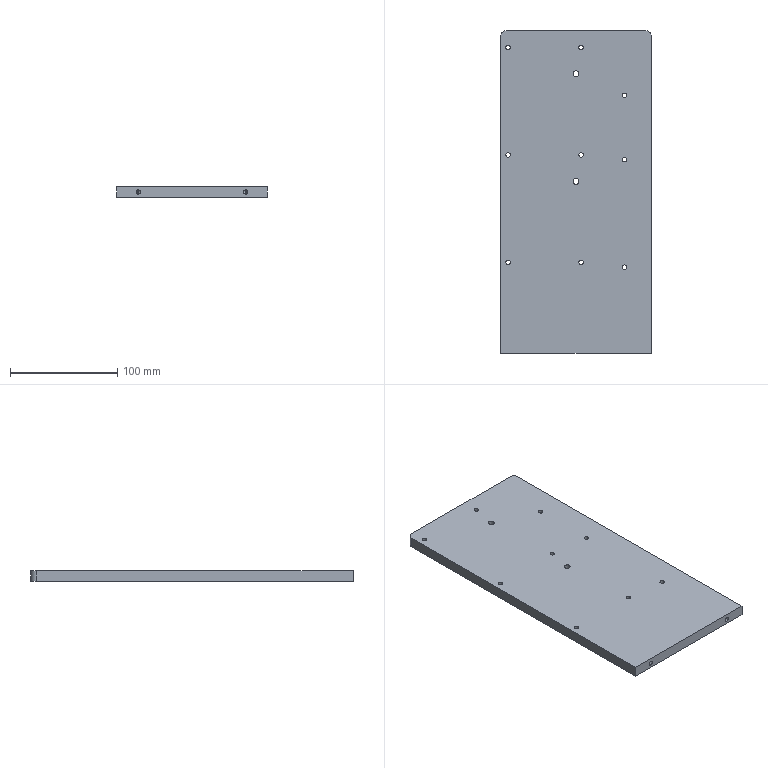Part | SolidWorks | features HoleWzd 4, Extrusion 1, Fillet 1 | 1 solid | 44 faces | box 140 x 300 x 10 mm | volume 417191 mm3 | cylinder 32 | plane 8 | cone 4 | commonest cylinder face diameters 4.2 x22 10 x6 5.5 x4
STEP:
#1=CARTESIAN_POINT('',(42.9,90.,0.));
#2=VERTEX_POINT('',#1);
#3=CARTESIAN_POINT('',(47.1,90.,0.));
#4=VERTEX_POINT('',#3);
#5=CARTESIAN_POINT('',(45.,90.,0.));
#6=DIRECTION('',(0.,0.,1.));
#7=DIRECTION('',(1.,0.,0.));
#8=AXIS2_PLACEMENT_3D('',#5,#6,#7);
#9=CIRCLE('',#8,2.1);
#10=EDGE_CURVE('',#2,#4,#9,.T.);
#11=ORIENTED_EDGE('',*,*,#10,.F.);
#12=CARTESIAN_POINT('',(42.9,90.,10.));
#13=VERTEX_POINT('',#12);
#14=CARTESIAN_POINT('',(42.9,90.,10.));
#15=DIRECTION('',(0.,0.,1.));
#16=VECTOR('',#15,1000.);
#17=LINE('',#14,#16);
#18=EDGE_CURVE('',#2,#13,#17,.T.);
#19=ORIENTED_EDGE('',*,*,#18,.T.);
#20=CARTESIAN_POINT('',(47.1,90.,10.));
#21=VERTEX_POINT('',#20);
#22=CARTESIAN_POINT('',(45.,90.,10.));
#23=DIRECTION('',(0.,0.,1.));
#24=DIRECTION('',(1.,0.,0.));
#25=AXIS2_PLACEMENT_3D('',#22,#23,#24);
#26=CIRCLE('',#25,2.1);
#27=EDGE_CURVE('',#13,#21,#26,.T.);
#28=ORIENTED_EDGE('',*,*,#27,.T.);
#29=CARTESIAN_POINT('',(47.1,90.,10.));
#30=DIRECTION('',(0.,0.,1.));
#31=VECTOR('',#30,1000.);
#32=LINE('',#29,#31);
#33=EDGE_CURVE('',#4,#21,#32,.T.);
#34=ORIENTED_EDGE('',*,*,#33,.F.);
#35=EDGE_LOOP('',(#11,#19,#28,#34));
#36=FACE_OUTER_BOUND('',#35,.T.);
#37=CARTESIAN_POINT('',(45.,90.,10.));
#38=DIRECTION('',(0.,0.,1.));
#39=DIRECTION('',(1.,0.,0.));
#40=AXIS2_PLACEMENT_3D('',#37,#38,#39);
#41=CYLINDRICAL_SURFACE('',#40,2.1);
#42=ADVANCED_FACE('',(#36),#41,.F.);
#43=CARTESIAN_POINT('',(42.9,30.,0.));
#44=VERTEX_POINT('',#43);
#45=CARTESIAN_POINT('',(47.1,30.,0.));
#46=VERTEX_POINT('',#45);
#47=CARTESIAN_POINT('',(45.,30.,0.));
#48=DIRECTION('',(0.,0.,1.));
#49=DIRECTION('',(1.,0.,0.));
#50=AXIS2_PLACEMENT_3D('',#47,#48,#49);
#51=CIRCLE('',#50,2.1);
#52=EDGE_CURVE('',#44,#46,#51,.T.);
#53=ORIENTED_EDGE('',*,*,#52,.F.);
#54=CARTESIAN_POINT('',(42.9,30.,10.));
#55=VERTEX_POINT('',#54);
#56=CARTESIAN_POINT('',(42.9,30.,10.));
#57=DIRECTION('',(0.,0.,1.));
#58=VECTOR('',#57,1000.);
#59=LINE('',#56,#58);
#60=EDGE_CURVE('',#44,#55,#59,.T.);
#61=ORIENTED_EDGE('',*,*,#60,.T.);
#62=CARTESIAN_POINT('',(47.1,30.,10.));
#63=VERTEX_POINT('',#62);
#64=CARTESIAN_POINT('',(45.,30.,10.));
#65=DIRECTION('',(0.,0.,1.));
#66=DIRECTION('',(1.,0.,0.));
#67=AXIS2_PLACEMENT_3D('',#64,#65,#66);
#68=CIRCLE('',#67,2.1);
#69=EDGE_CURVE('',#55,#63,#68,.T.);
#70=ORIENTED_EDGE('',*,*,#69,.T.);
#71=CARTESIAN_POINT('',(47.1,30.,10.));
#72=DIRECTION('',(0.,0.,1.));
#73=VECTOR('',#72,1000.);
#74=LINE('',#71,#73);
#75=EDGE_CURVE('',#46,#63,#74,.T.);
#76=ORIENTED_EDGE('',*,*,#75,.F.);
#77=EDGE_LOOP('',(#53,#61,#70,#76));
#78=FACE_OUTER_BOUND('',#77,.T.);
#79=CARTESIAN_POINT('',(45.,30.,10.));
#80=DIRECTION('',(0.,0.,1.));
#81=DIRECTION('',(1.,0.,0.));
#82=AXIS2_PLACEMENT_3D('',#79,#80,#81);
#83=CYLINDRICAL_SURFACE('',#82,2.1);
#84=ADVANCED_FACE('',(#78),#83,.F.);
#85=CARTESIAN_POINT('',(42.9,-70.,0.));
#86=VERTEX_POINT('',#85);
#87=CARTESIAN_POINT('',(47.1,-70.,0.));
#88=VERTEX_POINT('',#87);
#89=CARTESIAN_POINT('',(45.,-70.,0.));
#90=DIRECTION('',(0.,0.,1.));
#91=DIRECTION('',(1.,0.,0.));
#92=AXIS2_PLACEMENT_3D('',#89,#90,#91);
#93=CIRCLE('',#92,2.1);
#94=EDGE_CURVE('',#86,#88,#93,.T.);
#95=ORIENTED_EDGE('',*,*,#94,.F.);
#96=CARTESIAN_POINT('',(42.9,-70.,10.));
#97=VERTEX_POINT('',#96);
#98=CARTESIAN_POINT('',(42.9,-70.,10.));
#99=DIRECTION('',(0.,0.,1.));
#100=VECTOR('',#99,1000.);
#101=LINE('',#98,#100);
#102=EDGE_CURVE('',#86,#97,#101,.T.);
#103=ORIENTED_EDGE('',*,*,#102,.T.);
#104=CARTESIAN_POINT('',(47.1,-70.,10.));
#105=VERTEX_POINT('',#104);
#106=CARTESIAN_POINT('',(45.,-70.,10.));
#107=DIRECTION('',(0.,0.,1.));
#108=DIRECTION('',(1.,0.,0.));
#109=AXIS2_PLACEMENT_3D('',#106,#107,#108);
#110=CIRCLE('',#109,2.1);
#111=EDGE_CURVE('',#97,#105,#110,.T.);
#112=ORIENTED_EDGE('',*,*,#111,.T.);
#113=CARTESIAN_POINT('',(47.1,-70.,10.));
#114=DIRECTION('',(0.,0.,1.));
#115=VECTOR('',#114,1000.);
#116=LINE('',#113,#115);
#117=EDGE_CURVE('',#88,#105,#116,.T.);
#118=ORIENTED_EDGE('',*,*,#117,.F.);
#119=EDGE_LOOP('',(#95,#103,#112,#118));
#120=FACE_OUTER_BOUND('',#119,.T.);
#121=CARTESIAN_POINT('',(45.,-70.,10.));
#122=DIRECTION('',(0.,0.,1.));
#123=DIRECTION('',(1.,0.,0.));
#124=AXIS2_PLACEMENT_3D('',#121,#122,#123);
#125=CYLINDRICAL_SURFACE('',#124,2.1);
#126=ADVANCED_FACE('',(#120),#125,.F.);
#127=CARTESIAN_POINT('',(50.,-137.6,7.1));
#128=VERTEX_POINT('',#127);
#129=CARTESIAN_POINT('',(50.,-137.6,2.9));
#130=VERTEX_POINT('',#129);
#131=CARTESIAN_POINT('',(50.,-137.6,5.));
#132=DIRECTION('',(0.,-1.,0.));
#133=DIRECTION('',(0.,0.,-1.));
#134=AXIS2_PLACEMENT_3D('',#131,#132,#133);
#135=CIRCLE('',#134,2.1);
#136=EDGE_CURVE('',#128,#130,#135,.T.);
#137=ORIENTED_EDGE('',*,*,#136,.F.);
#138=CARTESIAN_POINT('',(50.,-150.,7.1));
#139=VERTEX_POINT('',#138);
#140=CARTESIAN_POINT('',(50.,-150.,7.1));
#141=DIRECTION('',(0.,-1.,0.));
#142=VECTOR('',#141,1000.);
#143=LINE('',#140,#142);
#144=EDGE_CURVE('',#128,#139,#143,.T.);
#145=ORIENTED_EDGE('',*,*,#144,.T.);
#146=CARTESIAN_POINT('',(50.,-150.,2.9));
#147=VERTEX_POINT('',#146);
#148=CARTESIAN_POINT('',(50.,-150.,5.));
#149=DIRECTION('',(0.,-1.,0.));
#150=DIRECTION('',(0.,0.,-1.));
#151=AXIS2_PLACEMENT_3D('',#148,#149,#150);
#152=CIRCLE('',#151,2.1);
#153=EDGE_CURVE('',#139,#147,#152,.T.);
#154=ORIENTED_EDGE('',*,*,#153,.T.);
#155=CARTESIAN_POINT('',(50.,-150.,2.9));
#156=DIRECTION('',(0.,-1.,0.));
#157=VECTOR('',#156,1000.);
#158=LINE('',#155,#157);
#159=EDGE_CURVE('',#130,#147,#158,.T.);
#160=ORIENTED_EDGE('',*,*,#159,.F.);
#161=EDGE_LOOP('',(#137,#145,#154,#160));
#162=FACE_OUTER_BOUND('',#161,.T.);
#163=CARTESIAN_POINT('',(50.,-150.,5.));
#164=DIRECTION('',(0.,-1.,0.));
#165=DIRECTION('',(0.,0.,-1.));
#166=AXIS2_PLACEMENT_3D('',#163,#164,#165);
#167=CYLINDRICAL_SURFACE('',#166,2.1);
#168=ADVANCED_FACE('',(#162),#167,.F.);
#169=CARTESIAN_POINT('',(50.,-136.338,5.));
#170=VERTEX_POINT('',#169);
#171=CARTESIAN_POINT('',(50.,-137.6,2.9));
#172=DIRECTION('',(0.,-0.515,-0.8572));
#173=VECTOR('',#172,1000.);
#174=LINE('',#171,#173);
#175=EDGE_CURVE('',#170,#130,#174,.T.);
#176=ORIENTED_EDGE('',*,*,#175,.F.);
#177=CARTESIAN_POINT('',(50.,-137.6,7.1));
#178=DIRECTION('',(0.,-0.515,0.8572));
#179=VECTOR('',#178,1000.);
#180=LINE('',#177,#179);
#181=EDGE_CURVE('',#170,#128,#180,.T.);
#182=ORIENTED_EDGE('',*,*,#181,.T.);
#183=ORIENTED_EDGE('',*,*,#136,.T.);
#184=EDGE_LOOP('',(#176,#182,#183));
#185=FACE_OUTER_BOUND('',#184,.T.);
#186=CARTESIAN_POINT('',(50.,-137.6,5.));
#187=DIRECTION('',(0.,-1.,0.));
#188=DIRECTION('',(0.,0.,-1.));
#189=AXIS2_PLACEMENT_3D('',#186,#187,#188);
#190=CONICAL_SURFACE('',#189,2.1,1.03);
#191=ADVANCED_FACE('',(#185),#190,.F.);
#192=CARTESIAN_POINT('',(-50.,-137.6,7.1));
#193=VERTEX_POINT('',#192);
#194=CARTESIAN_POINT('',(-50.,-137.6,2.9));
#195=VERTEX_POINT('',#194);
#196=CARTESIAN_POINT('',(-50.,-137.6,5.));
#197=DIRECTION('',(0.,-1.,0.));
#198=DIRECTION('',(0.,0.,-1.));
#199=AXIS2_PLACEMENT_3D('',#196,#197,#198);
#200=CIRCLE('',#199,2.1);
#201=EDGE_CURVE('',#193,#195,#200,.T.);
#202=ORIENTED_EDGE('',*,*,#201,.F.);
#203=CARTESIAN_POINT('',(-50.,-150.,7.1));
#204=VERTEX_POINT('',#203);
#205=CARTESIAN_POINT('',(-50.,-150.,7.1));
#206=DIRECTION('',(0.,-1.,0.));
#207=VECTOR('',#206,1000.);
#208=LINE('',#205,#207);
#209=EDGE_CURVE('',#193,#204,#208,.T.);
#210=ORIENTED_EDGE('',*,*,#209,.T.);
#211=CARTESIAN_POINT('',(-50.,-150.,2.9));
#212=VERTEX_POINT('',#211);
#213=CARTESIAN_POINT('',(-50.,-150.,5.));
#214=DIRECTION('',(0.,-1.,0.));
#215=DIRECTION('',(0.,0.,-1.));
#216=AXIS2_PLACEMENT_3D('',#213,#214,#215);
#217=CIRCLE('',#216,2.1);
#218=EDGE_CURVE('',#204,#212,#217,.T.);
#219=ORIENTED_EDGE('',*,*,#218,.T.);
#220=CARTESIAN_POINT('',(-50.,-150.,2.9));
#221=DIRECTION('',(0.,-1.,0.));
#222=VECTOR('',#221,1000.);
#223=LINE('',#220,#222);
#224=EDGE_CURVE('',#195,#212,#223,.T.);
#225=ORIENTED_EDGE('',*,*,#224,.F.);
#226=EDGE_LOOP('',(#202,#210,#219,#225));
#227=FACE_OUTER_BOUND('',#226,.T.);
#228=CARTESIAN_POINT('',(-50.,-150.,5.));
#229=DIRECTION('',(0.,-1.,0.));
#230=DIRECTION('',(0.,0.,-1.));
#231=AXIS2_PLACEMENT_3D('',#228,#229,#230);
#232=CYLINDRICAL_SURFACE('',#231,2.1);
#233=ADVANCED_FACE('',(#227),#232,.F.);
#234=CARTESIAN_POINT('',(-50.,-136.338,5.));
#235=VERTEX_POINT('',#234);
#236=CARTESIAN_POINT('',(-50.,-137.6,2.9));
#237=DIRECTION('',(0.,-0.515,-0.8572));
#238=VECTOR('',#237,1000.);
#239=LINE('',#236,#238);
#240=EDGE_CURVE('',#235,#195,#239,.T.);
#241=ORIENTED_EDGE('',*,*,#240,.F.);
#242=CARTESIAN_POINT('',(-50.,-137.6,7.1));
#243=DIRECTION('',(0.,-0.515,0.8572));
#244=VECTOR('',#243,1000.);
#245=LINE('',#242,#244);
#246=EDGE_CURVE('',#235,#193,#245,.T.);
#247=ORIENTED_EDGE('',*,*,#246,.T.);
#248=ORIENTED_EDGE('',*,*,#201,.T.);
#249=EDGE_LOOP('',(#241,#247,#248));
#250=FACE_OUTER_BOUND('',#249,.T.);
#251=CARTESIAN_POINT('',(-50.,-137.6,5.));
#252=DIRECTION('',(0.,-1.,0.));
#253=DIRECTION('',(0.,0.,-1.));
#254=AXIS2_PLACEMENT_3D('',#251,#252,#253);
#255=CONICAL_SURFACE('',#254,2.1,1.03);
#256=ADVANCED_FACE('',(#250),#255,.F.);
#257=CARTESIAN_POINT('',(2.7,-65.5,10.));
#258=VERTEX_POINT('',#257);
#259=CARTESIAN_POINT('',(6.9,-65.5,10.));
#260=VERTEX_POINT('',#259);
#261=CARTESIAN_POINT('',(4.8,-65.5,10.));
#262=DIRECTION('',(0.,0.,1.));
#263=DIRECTION('',(1.,0.,0.));
#264=AXIS2_PLACEMENT_3D('',#261,#262,#263);
#265=CIRCLE('',#264,2.1);
#266=EDGE_CURVE('',#258,#260,#265,.T.);
#267=ORIENTED_EDGE('',*,*,#266,.T.);
#268=CARTESIAN_POINT('',(6.9,-65.5,0.));
#269=VERTEX_POINT('',#268);
#270=CARTESIAN_POINT('',(6.9,-65.5,0.));
#271=DIRECTION('',(0.,0.,-1.));
#272=VECTOR('',#271,1000.);
#273=LINE('',#270,#272);
#274=EDGE_CURVE('',#260,#269,#273,.T.);
#275=ORIENTED_EDGE('',*,*,#274,.T.);
#276=CARTESIAN_POINT('',(2.7,-65.5,0.));
#277=VERTEX_POINT('',#276);
#278=CARTESIAN_POINT('',(4.8,-65.5,0.));
#279=DIRECTION('',(0.,0.,-1.));
#280=DIRECTION('',(-1.,0.,0.));
#281=AXIS2_PLACEMENT_3D('',#278,#279,#280);
#282=CIRCLE('',#281,2.1);
#283=EDGE_CURVE('',#269,#277,#282,.T.);
#284=ORIENTED_EDGE('',*,*,#283,.T.);
#285=CARTESIAN_POINT('',(2.7,-65.5,0.));
#286=DIRECTION('',(0.,0.,-1.));
#287=VECTOR('',#286,1000.);
#288=LINE('',#285,#287);
#289=EDGE_CURVE('',#258,#277,#288,.T.);
#290=ORIENTED_EDGE('',*,*,#289,.F.);
#291=EDGE_LOOP('',(#267,#275,#284,#290));
#292=FACE_OUTER_BOUND('',#291,.T.);
#293=CARTESIAN_POINT('',(4.8,-65.5,0.));
#294=DIRECTION('',(0.,0.,-1.));
#295=DIRECTION('',(-1.,0.,0.));
#296=AXIS2_PLACEMENT_3D('',#293,#294,#295);
#297=CYLINDRICAL_SURFACE('',#296,2.1);
#298=ADVANCED_FACE('',(#292),#297,.F.);
#299=CARTESIAN_POINT('',(-65.3,-65.5,10.));
#300=VERTEX_POINT('',#299);
#301=CARTESIAN_POINT('',(-61.1,-65.5,10.));
#302=VERTEX_POINT('',#301);
#303=CARTESIAN_POINT('',(-63.2,-65.5,10.));
#304=DIRECTION('',(0.,0.,1.));
#305=DIRECTION('',(1.,0.,0.));
#306=AXIS2_PLACEMENT_3D('',#303,#304,#305);
#307=CIRCLE('',#306,2.1);
#308=EDGE_CURVE('',#300,#302,#307,.T.);
#309=ORIENTED_EDGE('',*,*,#308,.T.);
#310=CARTESIAN_POINT('',(-61.1,-65.5,0.));
#311=VERTEX_POINT('',#310);
#312=CARTESIAN_POINT('',(-61.1,-65.5,0.));
#313=DIRECTION('',(0.,0.,-1.));
#314=VECTOR('',#313,1000.);
#315=LINE('',#312,#314);
#316=EDGE_CURVE('',#302,#311,#315,.T.);
#317=ORIENTED_EDGE('',*,*,#316,.T.);
#318=CARTESIAN_POINT('',(-65.3,-65.5,0.));
#319=VERTEX_POINT('',#318);
#320=CARTESIAN_POINT('',(-63.2,-65.5,0.));
#321=DIRECTION('',(0.,0.,-1.));
#322=DIRECTION('',(-1.,0.,0.));
#323=AXIS2_PLACEMENT_3D('',#320,#321,#322);
#324=CIRCLE('',#323,2.1);
#325=EDGE_CURVE('',#311,#319,#324,.T.);
#326=ORIENTED_EDGE('',*,*,#325,.T.);
#327=CARTESIAN_POINT('',(-65.3,-65.5,0.));
#328=DIRECTION('',(0.,0.,-1.));
#329=VECTOR('',#328,1000.);
#330=LINE('',#327,#329);
#331=EDGE_CURVE('',#300,#319,#330,.T.);
#332=ORIENTED_EDGE('',*,*,#331,.F.);
#333=EDGE_LOOP('',(#309,#317,#326,#332));
#334=FACE_OUTER_BOUND('',#333,.T.);
#335=CARTESIAN_POINT('',(-63.2,-65.5,0.));
#336=DIRECTION('',(0.,0.,-1.));
#337=DIRECTION('',(-1.,0.,0.));
#338=AXIS2_PLACEMENT_3D('',#335,#336,#337);
#339=CYLINDRICAL_SURFACE('',#338,2.1);
#340=ADVANCED_FACE('',(#334),#339,.F.);
#341=CARTESIAN_POINT('',(2.7,34.5,10.));
#342=VERTEX_POINT('',#341);
#343=CARTESIAN_POINT('',(6.9,34.5,10.));
#344=VERTEX_POINT('',#343);
#345=CARTESIAN_POINT('',(4.8,34.5,10.));
#346=DIRECTION('',(0.,0.,1.));
#347=DIRECTION('',(1.,0.,0.));
#348=AXIS2_PLACEMENT_3D('',#345,#346,#347);
#349=CIRCLE('',#348,2.1);
#350=EDGE_CURVE('',#342,#344,#349,.T.);
#351=ORIENTED_EDGE('',*,*,#350,.T.);
#352=CARTESIAN_POINT('',(6.9,34.5,0.));
#353=VERTEX_POINT('',#352);
#354=CARTESIAN_POINT('',(6.9,34.5,0.));
#355=DIRECTION('',(0.,0.,-1.));
#356=VECTOR('',#355,1000.);
#357=LINE('',#354,#356);
#358=EDGE_CURVE('',#344,#353,#357,.T.);
#359=ORIENTED_EDGE('',*,*,#358,.T.);
#360=CARTESIAN_POINT('',(2.7,34.5,0.));
#361=VERTEX_POINT('',#360);
#362=CARTESIAN_POINT('',(4.8,34.5,0.));
#363=DIRECTION('',(0.,0.,-1.));
#364=DIRECTION('',(-1.,0.,0.));
#365=AXIS2_PLACEMENT_3D('',#362,#363,#364);
#366=CIRCLE('',#365,2.1);
#367=EDGE_CURVE('',#353,#361,#366,.T.);
#368=ORIENTED_EDGE('',*,*,#367,.T.);
#369=CARTESIAN_POINT('',(2.7,34.5,0.));
#370=DIRECTION('',(0.,0.,-1.));
#371=VECTOR('',#370,1000.);
#372=LINE('',#369,#371);
#373=EDGE_CURVE('',#342,#361,#372,.T.);
#374=ORIENTED_EDGE('',*,*,#373,.F.);
#375=EDGE_LOOP('',(#351,#359,#368,#374));
#376=FACE_OUTER_BOUND('',#375,.T.);
#377=CARTESIAN_POINT('',(4.8,34.5,0.));
#378=DIRECTION('',(0.,0.,-1.));
#379=DIRECTION('',(-1.,0.,0.));
#380=AXIS2_PLACEMENT_3D('',#377,#378,#379);
#381=CYLINDRICAL_SURFACE('',#380,2.1);
#382=ADVANCED_FACE('',(#376),#381,.F.);
#383=CARTESIAN_POINT('',(-65.3,34.5,10.));
#384=VERTEX_POINT('',#383);
#385=CARTESIAN_POINT('',(-61.1,34.5,10.));
#386=VERTEX_POINT('',#385);
#387=CARTESIAN_POINT('',(-63.2,34.5,10.));
#388=DIRECTION('',(0.,0.,1.));
#389=DIRECTION('',(1.,0.,0.));
#390=AXIS2_PLACEMENT_3D('',#387,#388,#389);
#391=CIRCLE('',#390,2.1);
#392=EDGE_CURVE('',#384,#386,#391,.T.);
#393=ORIENTED_EDGE('',*,*,#392,.T.);
#394=CARTESIAN_POINT('',(-61.1,34.5,0.));
#395=VERTEX_POINT('',#394);
#396=CARTESIAN_POINT('',(-61.1,34.5,0.));
#397=DIRECTION('',(0.,0.,-1.));
#398=VECTOR('',#397,1000.);
#399=LINE('',#396,#398);
#400=EDGE_CURVE('',#386,#395,#399,.T.);
#401=ORIENTED_EDGE('',*,*,#400,.T.);
#402=CARTESIAN_POINT('',(-65.3,34.5,0.));
#403=VERTEX_POINT('',#402);
#404=CARTESIAN_POINT('',(-63.2,34.5,0.));
#405=DIRECTION('',(0.,0.,-1.));
#406=DIRECTION('',(-1.,0.,0.));
#407=AXIS2_PLACEMENT_3D('',#404,#405,#406);
#408=CIRCLE('',#407,2.1);
#409=EDGE_CURVE('',#395,#403,#408,.T.);
#410=ORIENTED_EDGE('',*,*,#409,.T.);
#411=CARTESIAN_POINT('',(-65.3,34.5,0.));
#412=DIRECTION('',(0.,0.,-1.));
#413=VECTOR('',#412,1000.);
#414=LINE('',#411,#413);
#415=EDGE_CURVE('',#384,#403,#414,.T.);
#416=ORIENTED_EDGE('',*,*,#415,.F.);
#417=EDGE_LOOP('',(#393,#401,#410,#416));
#418=FACE_OUTER_BOUND('',#417,.T.);
#419=CARTESIAN_POINT('',(-63.2,34.5,0.));
#420=DIRECTION('',(0.,0.,-1.));
#421=DIRECTION('',(-1.,0.,0.));
#422=AXIS2_PLACEMENT_3D('',#419,#420,#421);
#423=CYLINDRICAL_SURFACE('',#422,2.1);
#424=ADVANCED_FACE('',(#418),#423,.F.);
#425=CARTESIAN_POINT('',(2.7,134.5,10.));
#426=VERTEX_POINT('',#425);
#427=CARTESIAN_POINT('',(6.9,134.5,10.));
#428=VERTEX_POINT('',#427);
#429=CARTESIAN_POINT('',(4.8,134.5,10.));
#430=DIRECTION('',(0.,0.,1.));
#431=DIRECTION('',(1.,0.,0.));
#432=AXIS2_PLACEMENT_3D('',#429,#430,#431);
#433=CIRCLE('',#432,2.1);
#434=EDGE_CURVE('',#426,#428,#433,.T.);
#435=ORIENTED_EDGE('',*,*,#434,.T.);
#436=CARTESIAN_POINT('',(6.9,134.5,0.));
#437=VERTEX_POINT('',#436);
#438=CARTESIAN_POINT('',(6.9,134.5,0.));
#439=DIRECTION('',(0.,0.,-1.));
#440=VECTOR('',#439,1000.);
#441=LINE('',#438,#440);
#442=EDGE_CURVE('',#428,#437,#441,.T.);
#443=ORIENTED_EDGE('',*,*,#442,.T.);
#444=CARTESIAN_POINT('',(2.7,134.5,0.));
#445=VERTEX_POINT('',#444);
#446=CARTESIAN_POINT('',(4.8,134.5,0.));
#447=DIRECTION('',(0.,0.,-1.));
#448=DIRECTION('',(-1.,0.,0.));
#449=AXIS2_PLACEMENT_3D('',#446,#447,#448);
#450=CIRCLE('',#449,2.1);
#451=EDGE_CURVE('',#437,#445,#450,.T.);
#452=ORIENTED_EDGE('',*,*,#451,.T.);
#453=CARTESIAN_POINT('',(2.7,134.5,0.));
#454=DIRECTION('',(0.,0.,-1.));
#455=VECTOR('',#454,1000.);
#456=LINE('',#453,#455);
#457=EDGE_CURVE('',#426,#445,#456,.T.);
#458=ORIENTED_EDGE('',*,*,#457,.F.);
#459=EDGE_LOOP('',(#435,#443,#452,#458));
#460=FACE_OUTER_BOUND('',#459,.T.);
#461=CARTESIAN_POINT('',(4.8,134.5,0.));
#462=DIRECTION('',(0.,0.,-1.));
#463=DIRECTION('',(-1.,0.,0.));
#464=AXIS2_PLACEMENT_3D('',#461,#462,#463);
#465=CYLINDRICAL_SURFACE('',#464,2.1);
#466=ADVANCED_FACE('',(#460),#465,.F.);
#467=CARTESIAN_POINT('',(-65.3,134.5,10.));
#468=VERTEX_POINT('',#467);
#469=CARTESIAN_POINT('',(-61.1,134.5,10.));
#470=VERTEX_POINT('',#469);
#471=CARTESIAN_POINT('',(-63.2,134.5,10.));
#472=DIRECTION('',(0.,0.,1.));
#473=DIRECTION('',(1.,0.,0.));
#474=AXIS2_PLACEMENT_3D('',#471,#472,#473);
#475=CIRCLE('',#474,2.1);
#476=EDGE_CURVE('',#468,#470,#475,.T.);
#477=ORIENTED_EDGE('',*,*,#476,.T.);
#478=CARTESIAN_POINT('',(-61.1,134.5,0.));
#479=VERTEX_POINT('',#478);
#480=CARTESIAN_POINT('',(-61.1,134.5,0.));
#481=DIRECTION('',(0.,0.,-1.));
#482=VECTOR('',#481,1000.);
#483=LINE('',#480,#482);
#484=EDGE_CURVE('',#470,#479,#483,.T.);
#485=ORIENTED_EDGE('',*,*,#484,.T.);
#486=CARTESIAN_POINT('',(-65.3,134.5,0.));
#487=VERTEX_POINT('',#486);
#488=CARTESIAN_POINT('',(-63.2,134.5,0.));
#489=DIRECTION('',(0.,0.,-1.));
#490=DIRECTION('',(-1.,0.,0.));
#491=AXIS2_PLACEMENT_3D('',#488,#489,#490);
#492=CIRCLE('',#491,2.1);
#493=EDGE_CURVE('',#479,#487,#492,.T.);
#494=ORIENTED_EDGE('',*,*,#493,.T.);
#495=CARTESIAN_POINT('',(-65.3,134.5,0.));
#496=DIRECTION('',(0.,0.,-1.));
#497=VECTOR('',#496,1000.);
#498=LINE('',#495,#497);
#499=EDGE_CURVE('',#468,#487,#498,.T.);
#500=ORIENTED_EDGE('',*,*,#499,.F.);
#501=EDGE_LOOP('',(#477,#485,#494,#500));
#502=FACE_OUTER_BOUND('',#501,.T.);
#503=CARTESIAN_POINT('',(-63.2,134.5,0.));
#504=DIRECTION('',(0.,0.,-1.));
#505=DIRECTION('',(-1.,0.,0.));
#506=AXIS2_PLACEMENT_3D('',#503,#504,#505);
#507=CYLINDRICAL_SURFACE('',#506,2.1);
#508=ADVANCED_FACE('',(#502),#507,.F.);
#509=CARTESIAN_POINT('',(5.,110.,5.7));
#510=VERTEX_POINT('',#509);
#511=CARTESIAN_POINT('',(-5.,110.,5.7));
#512=VERTEX_POINT('',#511);
#513=CARTESIAN_POINT('',(0.,110.,5.7));
#514=DIRECTION('',(0.,0.,-1.));
#515=DIRECTION('',(-1.,0.,0.));
#516=AXIS2_PLACEMENT_3D('',#513,#514,#515);
#517=CIRCLE('',#516,5.);
#518=EDGE_CURVE('',#510,#512,#517,.T.);
#519=ORIENTED_EDGE('',*,*,#518,.F.);
#520=CARTESIAN_POINT('',(5.,110.,0.));
#521=VERTEX_POINT('',#520);
#522=CARTESIAN_POINT('',(5.,110.,0.));
#523=DIRECTION('',(0.,0.,-1.));
#524=VECTOR('',#523,1000.);
#525=LINE('',#522,#524);
#526=EDGE_CURVE('',#510,#521,#525,.T.);
#527=ORIENTED_EDGE('',*,*,#526,.T.);
#528=CARTESIAN_POINT('',(-5.,110.,0.));
#529=VERTEX_POINT('',#528);
#530=CARTESIAN_POINT('',(0.,110.,0.));
#531=DIRECTION('',(0.,0.,-1.));
#532=DIRECTION('',(-1.,0.,0.));
#533=AXIS2_PLACEMENT_3D('',#530,#531,#532);
#534=CIRCLE('',#533,5.);
#535=EDGE_CURVE('',#521,#529,#534,.T.);
#536=ORIENTED_EDGE('',*,*,#535,.T.);
#537=CARTESIAN_POINT('',(-5.,110.,0.));
#538=DIRECTION('',(0.,0.,-1.));
#539=VECTOR('',#538,1000.);
#540=LINE('',#537,#539);
#541=EDGE_CURVE('',#512,#529,#540,.T.);
#542=ORIENTED_EDGE('',*,*,#541,.F.);
#543=EDGE_LOOP('',(#519,#527,#536,#542));
#544=FACE_OUTER_BOUND('',#543,.T.);
#545=CARTESIAN_POINT('',(0.,110.,0.));
#546=DIRECTION('',(0.,0.,-1.));
#547=DIRECTION('',(-1.,0.,0.));
#548=AXIS2_PLACEMENT_3D('',#545,#546,#547);
#549=CYLINDRICAL_SURFACE('',#548,5.);
#550=ADVANCED_FACE('',(#544),#549,.F.);
#551=CARTESIAN_POINT('',(-2.75,110.,10.));
#552=VERTEX_POINT('',#551);
#553=CARTESIAN_POINT('',(2.75,110.,10.));
#554=VERTEX_POINT('',#553);
#555=CARTESIAN_POINT('',(0.,110.,10.));
#556=DIRECTION('',(0.,0.,1.));
#557=DIRECTION('',(1.,0.,0.));
#558=AXIS2_PLACEMENT_3D('',#555,#556,#557);
#559=CIRCLE('',#558,2.75);
#560=EDGE_CURVE('',#552,#554,#559,.T.);
#561=ORIENTED_EDGE('',*,*,#560,.T.);
#562=CARTESIAN_POINT('',(2.75,110.,5.7));
#563=VERTEX_POINT('',#562);
#564=CARTESIAN_POINT('',(2.75,110.,0.));
#565=DIRECTION('',(0.,0.,-1.));
#566=VECTOR('',#565,1000.);
#567=LINE('',#564,#566);
#568=EDGE_CURVE('',#554,#563,#567,.T.);
#569=ORIENTED_EDGE('',*,*,#568,.T.);
#570=CARTESIAN_POINT('',(-2.75,110.,5.7));
#571=VERTEX_POINT('',#570);
#572=CARTESIAN_POINT('',(0.,110.,5.7));
#573=DIRECTION('',(0.,0.,-1.));
#574=DIRECTION('',(-1.,0.,0.));
#575=AXIS2_PLACEMENT_3D('',#572,#573,#574);
#576=CIRCLE('',#575,2.75);
#577=EDGE_CURVE('',#563,#571,#576,.T.);
#578=ORIENTED_EDGE('',*,*,#577,.T.);
#579=CARTESIAN_POINT('',(-2.75,110.,0.));
#580=DIRECTION('',(0.,0.,-1.));
#581=VECTOR('',#580,1000.);
#582=LINE('',#579,#581);
#583=EDGE_CURVE('',#552,#571,#582,.T.);
#584=ORIENTED_EDGE('',*,*,#583,.F.);
#585=EDGE_LOOP('',(#561,#569,#578,#584));
#586=FACE_OUTER_BOUND('',#585,.T.);
#587=CARTESIAN_POINT('',(0.,110.,0.));
#588=DIRECTION('',(0.,0.,-1.));
#589=DIRECTION('',(-1.,0.,0.));
#590=AXIS2_PLACEMENT_3D('',#587,#588,#589);
#591=CYLINDRICAL_SURFACE('',#590,2.75);
#592=ADVANCED_FACE('',(#586),#591,.F.);
#593=CARTESIAN_POINT('',(5.,10.,5.7));
#594=VERTEX_POINT('',#593);
#595=CARTESIAN_POINT('',(-5.,10.,5.7));
#596=VERTEX_POINT('',#595);
#597=CARTESIAN_POINT('',(0.,10.,5.7));
#598=DIRECTION('',(0.,0.,-1.));
#599=DIRECTION('',(-1.,0.,0.));
#600=AXIS2_PLACEMENT_3D('',#597,#598,#599);
#601=CIRCLE('',#600,5.);
#602=EDGE_CURVE('',#594,#596,#601,.T.);
#603=ORIENTED_EDGE('',*,*,#602,.F.);
#604=CARTESIAN_POINT('',(5.,10.,0.));
#605=VERTEX_POINT('',#604);
#606=CARTESIAN_POINT('',(5.,10.,0.));
#607=DIRECTION('',(0.,0.,-1.));
#608=VECTOR('',#607,1000.);
#609=LINE('',#606,#608);
#610=EDGE_CURVE('',#594,#605,#609,.T.);
#611=ORIENTED_EDGE('',*,*,#610,.T.);
#612=CARTESIAN_POINT('',(-5.,10.,0.));
#613=VERTEX_POINT('',#612);
#614=CARTESIAN_POINT('',(0.,10.,0.));
#615=DIRECTION('',(0.,0.,-1.));
#616=DIRECTION('',(-1.,0.,0.));
#617=AXIS2_PLACEMENT_3D('',#614,#615,#616);
#618=CIRCLE('',#617,5.);
#619=EDGE_CURVE('',#605,#613,#618,.T.);
#620=ORIENTED_EDGE('',*,*,#619,.T.);
#621=CARTESIAN_POINT('',(-5.,10.,0.));
#622=DIRECTION('',(0.,0.,-1.));
#623=VECTOR('',#622,1000.);
#624=LINE('',#621,#623);
#625=EDGE_CURVE('',#596,#613,#624,.T.);
#626=ORIENTED_EDGE('',*,*,#625,.F.);
#627=EDGE_LOOP('',(#603,#611,#620,#626));
#628=FACE_OUTER_BOUND('',#627,.T.);
#629=CARTESIAN_POINT('',(0.,10.,0.));
#630=DIRECTION('',(0.,0.,-1.));
#631=DIRECTION('',(-1.,0.,0.));
#632=AXIS2_PLACEMENT_3D('',#629,#630,#631);
#633=CYLINDRICAL_SURFACE('',#632,5.);
#634=ADVANCED_FACE('',(#628),#633,.F.);
#635=CARTESIAN_POINT('',(-2.75,10.,10.));
#636=VERTEX_POINT('',#635);
#637=CARTESIAN_POINT('',(2.75,10.,10.));
#638=VERTEX_POINT('',#637);
#639=CARTESIAN_POINT('',(0.,10.,10.));
#640=DIRECTION('',(0.,0.,1.));
#641=DIRECTION('',(1.,0.,0.));
#642=AXIS2_PLACEMENT_3D('',#639,#640,#641);
#643=CIRCLE('',#642,2.75);
#644=EDGE_CURVE('',#636,#638,#643,.T.);
#645=ORIENTED_EDGE('',*,*,#644,.T.);
#646=CARTESIAN_POINT('',(2.75,10.,5.7));
#647=VERTEX_POINT('',#646);
#648=CARTESIAN_POINT('',(2.75,10.,0.));
#649=DIRECTION('',(0.,0.,-1.));
#650=VECTOR('',#649,1000.);
#651=LINE('',#648,#650);
#652=EDGE_CURVE('',#638,#647,#651,.T.);
#653=ORIENTED_EDGE('',*,*,#652,.T.);
#654=CARTESIAN_POINT('',(-2.75,10.,5.7));
#655=VERTEX_POINT('',#654);
#656=CARTESIAN_POINT('',(0.,10.,5.7));
#657=DIRECTION('',(0.,0.,-1.));
#658=DIRECTION('',(-1.,0.,0.));
#659=AXIS2_PLACEMENT_3D('',#656,#657,#658);
#660=CIRCLE('',#659,2.75);
#661=EDGE_CURVE('',#647,#655,#660,.T.);
#662=ORIENTED_EDGE('',*,*,#661,.T.);
#663=CARTESIAN_POINT('',(-2.75,10.,0.));
#664=DIRECTION('',(0.,0.,-1.));
#665=VECTOR('',#664,1000.);
#666=LINE('',#663,#665);
#667=EDGE_CURVE('',#636,#655,#666,.T.);
#668=ORIENTED_EDGE('',*,*,#667,.F.);
#669=EDGE_LOOP('',(#645,#653,#662,#668));
#670=FACE_OUTER_BOUND('',#669,.T.);
#671=CARTESIAN_POINT('',(0.,10.,0.));
#672=DIRECTION('',(0.,0.,-1.));
#673=DIRECTION('',(-1.,0.,0.));
#674=AXIS2_PLACEMENT_3D('',#671,#672,#673);
#675=CYLINDRICAL_SURFACE('',#674,2.75);
#676=ADVANCED_FACE('',(#670),#675,.F.);
#677=CARTESIAN_POINT('',(45.,90.,0.));
#678=DIRECTION('',(0.,0.,1.));
#679=DIRECTION('',(1.,0.,0.));
#680=AXIS2_PLACEMENT_3D('',#677,#678,#679);
#681=CIRCLE('',#680,2.1);
#682=EDGE_CURVE('',#4,#2,#681,.T.);
#683=ORIENTED_EDGE('',*,*,#682,.T.);
#684=ORIENTED_EDGE('',*,*,#10,.T.);
#685=EDGE_LOOP('',(#683,#684));
#686=FACE_BOUND('',#685,.T.);
#687=CARTESIAN_POINT('',(45.,30.,0.));
#688=DIRECTION('',(0.,0.,1.));
#689=DIRECTION('',(1.,0.,0.));
#690=AXIS2_PLACEMENT_3D('',#687,#688,#689);
#691=CIRCLE('',#690,2.1);
#692=EDGE_CURVE('',#46,#44,#691,.T.);
#693=ORIENTED_EDGE('',*,*,#692,.T.);
#694=ORIENTED_EDGE('',*,*,#52,.T.);
#695=EDGE_LOOP('',(#693,#694));
#696=FACE_BOUND('',#695,.T.);
#697=CARTESIAN_POINT('',(45.,-70.,0.));
#698=DIRECTION('',(0.,0.,1.));
#699=DIRECTION('',(1.,0.,0.));
#700=AXIS2_PLACEMENT_3D('',#697,#698,#699);
#701=CIRCLE('',#700,2.1);
#702=EDGE_CURVE('',#88,#86,#701,.T.);
#703=ORIENTED_EDGE('',*,*,#702,.T.);
#704=ORIENTED_EDGE('',*,*,#94,.T.);
#705=EDGE_LOOP('',(#703,#704));
#706=FACE_BOUND('',#705,.T.);
#707=CARTESIAN_POINT('',(4.8,-65.5,0.));
#708=DIRECTION('',(0.,0.,-1.));
#709=DIRECTION('',(-1.,0.,0.));
#710=AXIS2_PLACEMENT_3D('',#707,#708,#709);
#711=CIRCLE('',#710,2.1);
#712=EDGE_CURVE('',#277,#269,#711,.T.);
#713=ORIENTED_EDGE('',*,*,#712,.F.);
#714=ORIENTED_EDGE('',*,*,#283,.F.);
#715=EDGE_LOOP('',(#713,#714));
#716=FACE_BOUND('',#715,.T.);
#717=CARTESIAN_POINT('',(-63.2,-65.5,0.));
#718=DIRECTION('',(0.,0.,-1.));
#719=DIRECTION('',(-1.,0.,0.));
#720=AXIS2_PLACEMENT_3D('',#717,#718,#719);
#721=CIRCLE('',#720,2.1);
#722=EDGE_CURVE('',#319,#311,#721,.T.);
#723=ORIENTED_EDGE('',*,*,#722,.F.);
#724=ORIENTED_EDGE('',*,*,#325,.F.);
#725=EDGE_LOOP('',(#723,#724));
#726=FACE_BOUND('',#725,.T.);
#727=CARTESIAN_POINT('',(4.8,34.5,0.));
#728=DIRECTION('',(0.,0.,-1.));
#729=DIRECTION('',(-1.,0.,0.));
#730=AXIS2_PLACEMENT_3D('',#727,#728,#729);
#731=CIRCLE('',#730,2.1);
#732=EDGE_CURVE('',#361,#353,#731,.T.);
#733=ORIENTED_EDGE('',*,*,#732,.F.);
#734=ORIENTED_EDGE('',*,*,#367,.F.);
#735=EDGE_LOOP('',(#733,#734));
#736=FACE_BOUND('',#735,.T.);
#737=CARTESIAN_POINT('',(4.8,134.5,0.));
#738=DIRECTION('',(0.,0.,-1.));
#739=DIRECTION('',(-1.,0.,0.));
#740=AXIS2_PLACEMENT_3D('',#737,#738,#739);
#741=CIRCLE('',#740,2.1);
#742=EDGE_CURVE('',#445,#437,#741,.T.);
#743=ORIENTED_EDGE('',*,*,#742,.F.);
#744=ORIENTED_EDGE('',*,*,#451,.F.);
#745=EDGE_LOOP('',(#743,#744));
#746=FACE_BOUND('',#745,.T.);
#747=CARTESIAN_POINT('',(-63.2,134.5,0.));
#748=DIRECTION('',(0.,0.,-1.));
#749=DIRECTION('',(-1.,0.,0.));
#750=AXIS2_PLACEMENT_3D('',#747,#748,#749);
#751=CIRCLE('',#750,2.1);
#752=EDGE_CURVE('',#487,#479,#751,.T.);
#753=ORIENTED_EDGE('',*,*,#752,.F.);
#754=ORIENTED_EDGE('',*,*,#493,.F.);
#755=EDGE_LOOP('',(#753,#754));
#756=FACE_BOUND('',#755,.T.);
#757=CARTESIAN_POINT('',(0.,110.,0.));
#758=DIRECTION('',(0.,0.,-1.));
#759=DIRECTION('',(-1.,0.,0.));
#760=AXIS2_PLACEMENT_3D('',#757,#758,#759);
#761=CIRCLE('',#760,5.);
#762=EDGE_CURVE('',#529,#521,#761,.T.);
#763=ORIENTED_EDGE('',*,*,#762,.F.);
#764=ORIENTED_EDGE('',*,*,#535,.F.);
#765=EDGE_LOOP('',(#763,#764));
#766=FACE_BOUND('',#765,.T.);
#767=CARTESIAN_POINT('',(0.,10.,0.));
#768=DIRECTION('',(0.,0.,-1.));
#769=DIRECTION('',(-1.,0.,0.));
#770=AXIS2_PLACEMENT_3D('',#767,#768,#769);
#771=CIRCLE('',#770,5.);
#772=EDGE_CURVE('',#613,#605,#771,.T.);
#773=ORIENTED_EDGE('',*,*,#772,.F.);
#774=ORIENTED_EDGE('',*,*,#619,.F.);
#775=EDGE_LOOP('',(#773,#774));
#776=FACE_BOUND('',#775,.T.);
#777=CARTESIAN_POINT('',(-70.,145.,0.));
#778=VERTEX_POINT('',#777);
#779=CARTESIAN_POINT('',(-70.,-150.,0.));
#780=VERTEX_POINT('',#779);
#781=CARTESIAN_POINT('',(-70.,-150.,0.));
#782=DIRECTION('',(0.,-1.,0.));
#783=VECTOR('',#782,1000.);
#784=LINE('',#781,#783);
#785=EDGE_CURVE('',#778,#780,#784,.T.);
#786=ORIENTED_EDGE('',*,*,#785,.F.);
#787=CARTESIAN_POINT('',(-65.,150.,0.));
#788=VERTEX_POINT('',#787);
#789=CARTESIAN_POINT('',(-65.,145.,0.));
#790=DIRECTION('',(0.,0.,-1.));
#791=DIRECTION('',(1.,0.,0.));
#792=AXIS2_PLACEMENT_3D('',#789,#790,#791);
#793=CIRCLE('',#792,5.);
#794=EDGE_CURVE('',#778,#788,#793,.T.);
#795=ORIENTED_EDGE('',*,*,#794,.T.);
#796=CARTESIAN_POINT('',(65.,150.,0.));
#797=VERTEX_POINT('',#796);
#798=CARTESIAN_POINT('',(70.,150.,0.));
#799=DIRECTION('',(-1.,0.,0.));
#800=VECTOR('',#799,1000.);
#801=LINE('',#798,#800);
#802=EDGE_CURVE('',#797,#788,#801,.T.);
#803=ORIENTED_EDGE('',*,*,#802,.F.);
#804=CARTESIAN_POINT('',(70.,145.,0.));
#805=VERTEX_POINT('',#804);
#806=CARTESIAN_POINT('',(65.,145.,0.));
#807=DIRECTION('',(0.,0.,-1.));
#808=DIRECTION('',(1.,0.,0.));
#809=AXIS2_PLACEMENT_3D('',#806,#807,#808);
#810=CIRCLE('',#809,5.);
#811=EDGE_CURVE('',#797,#805,#810,.T.);
#812=ORIENTED_EDGE('',*,*,#811,.T.);
#813=CARTESIAN_POINT('',(70.,-150.,0.));
#814=VERTEX_POINT('',#813);
#815=CARTESIAN_POINT('',(70.,-150.,0.));
#816=DIRECTION('',(0.,1.,0.));
#817=VECTOR('',#816,1000.);
#818=LINE('',#815,#817);
#819=EDGE_CURVE('',#814,#805,#818,.T.);
#820=ORIENTED_EDGE('',*,*,#819,.F.);
#821=CARTESIAN_POINT('',(70.,-150.,0.));
#822=DIRECTION('',(1.,0.,0.));
#823=VECTOR('',#822,1000.);
#824=LINE('',#821,#823);
#825=EDGE_CURVE('',#780,#814,#824,.T.);
#826=ORIENTED_EDGE('',*,*,#825,.F.);
#827=EDGE_LOOP('',(#786,#795,#803,#812,#820,#826));
#828=FACE_OUTER_BOUND('',#827,.T.);
#829=CARTESIAN_POINT('',(-63.2,34.5,0.));
#830=DIRECTION('',(0.,0.,-1.));
#831=DIRECTION('',(-1.,0.,0.));
#832=AXIS2_PLACEMENT_3D('',#829,#830,#831);
#833=CIRCLE('',#832,2.1);
#834=EDGE_CURVE('',#403,#395,#833,.T.);
#835=ORIENTED_EDGE('',*,*,#834,.F.);
#836=ORIENTED_EDGE('',*,*,#409,.F.);
#837=EDGE_LOOP('',(#835,#836));
#838=FACE_BOUND('',#837,.T.);
#839=CARTESIAN_POINT('',(0.,0.,0.));
#840=DIRECTION('',(0.,0.,1.));
#841=DIRECTION('',(1.,0.,0.));
#842=AXIS2_PLACEMENT_3D('',#839,#840,#841);
#843=PLANE('',#842);
#844=ADVANCED_FACE('',(#686,#696,#706,#716,#726,#736,#746,#756,#766,#776,#828,#838),#843,.F.);
#845=CARTESIAN_POINT('',(-70.,145.,10.));
#846=VERTEX_POINT('',#845);
#847=CARTESIAN_POINT('',(-70.,-150.,10.));
#848=VERTEX_POINT('',#847);
#849=CARTESIAN_POINT('',(-70.,-150.,10.));
#850=DIRECTION('',(0.,-1.,0.));
#851=VECTOR('',#850,1000.);
#852=LINE('',#849,#851);
#853=EDGE_CURVE('',#846,#848,#852,.T.);
#854=ORIENTED_EDGE('',*,*,#853,.F.);
#855=CARTESIAN_POINT('',(-70.,145.,10.));
#856=DIRECTION('',(0.,0.,-1.));
#857=VECTOR('',#856,1000.);
#858=LINE('',#855,#857);
#859=EDGE_CURVE('',#846,#778,#858,.T.);
#860=ORIENTED_EDGE('',*,*,#859,.T.);
#861=ORIENTED_EDGE('',*,*,#785,.T.);
#862=CARTESIAN_POINT('',(-70.,-150.,10.));
#863=DIRECTION('',(0.,0.,-1.));
#864=VECTOR('',#863,1000.);
#865=LINE('',#862,#864);
#866=EDGE_CURVE('',#848,#780,#865,.T.);
#867=ORIENTED_EDGE('',*,*,#866,.F.);
#868=EDGE_LOOP('',(#854,#860,#861,#867));
#869=FACE_OUTER_BOUND('',#868,.T.);
#870=CARTESIAN_POINT('',(-70.,-150.,10.));
#871=DIRECTION('',(1.,0.,0.));
#872=DIRECTION('',(0.,0.,-1.));
#873=AXIS2_PLACEMENT_3D('',#870,#871,#872);
#874=PLANE('',#873);
#875=ADVANCED_FACE('',(#869),#874,.F.);
#876=CARTESIAN_POINT('',(50.,-150.,5.));
#877=DIRECTION('',(0.,-1.,0.));
#878=DIRECTION('',(0.,0.,-1.));
#879=AXIS2_PLACEMENT_3D('',#876,#877,#878);
#880=CIRCLE('',#879,2.1);
#881=EDGE_CURVE('',#147,#139,#880,.T.);
#882=ORIENTED_EDGE('',*,*,#881,.F.);
#883=ORIENTED_EDGE('',*,*,#153,.F.);
#884=EDGE_LOOP('',(#882,#883));
#885=FACE_BOUND('',#884,.T.);
#886=CARTESIAN_POINT('',(-50.,-150.,5.));
#887=DIRECTION('',(0.,-1.,0.));
#888=DIRECTION('',(0.,0.,-1.));
#889=AXIS2_PLACEMENT_3D('',#886,#887,#888);
#890=CIRCLE('',#889,2.1);
#891=EDGE_CURVE('',#212,#204,#890,.T.);
#892=ORIENTED_EDGE('',*,*,#891,.F.);
#893=ORIENTED_EDGE('',*,*,#218,.F.);
#894=EDGE_LOOP('',(#892,#893));
#895=FACE_BOUND('',#894,.T.);
#896=ORIENTED_EDGE('',*,*,#825,.T.);
#897=CARTESIAN_POINT('',(70.,-150.,10.));
#898=VERTEX_POINT('',#897);
#899=CARTESIAN_POINT('',(70.,-150.,10.));
#900=DIRECTION('',(0.,0.,-1.));
#901=VECTOR('',#900,1000.);
#902=LINE('',#899,#901);
#903=EDGE_CURVE('',#898,#814,#902,.T.);
#904=ORIENTED_EDGE('',*,*,#903,.F.);
#905=CARTESIAN_POINT('',(70.,-150.,10.));
#906=DIRECTION('',(1.,0.,0.));
#907=VECTOR('',#906,1000.);
#908=LINE('',#905,#907);
#909=EDGE_CURVE('',#848,#898,#908,.T.);
#910=ORIENTED_EDGE('',*,*,#909,.F.);
#911=ORIENTED_EDGE('',*,*,#866,.T.);
#912=EDGE_LOOP('',(#896,#904,#910,#911));
#913=FACE_OUTER_BOUND('',#912,.T.);
#914=CARTESIAN_POINT('',(70.,-150.,10.));
#915=DIRECTION('',(0.,1.,0.));
#916=DIRECTION('',(-1.,0.,0.));
#917=AXIS2_PLACEMENT_3D('',#914,#915,#916);
#918=PLANE('',#917);
#919=ADVANCED_FACE('',(#885,#895,#913),#918,.F.);
#920=ORIENTED_EDGE('',*,*,#819,.T.);
#921=CARTESIAN_POINT('',(70.,145.,10.));
#922=VERTEX_POINT('',#921);
#923=CARTESIAN_POINT('',(70.,145.,10.));
#924=DIRECTION('',(0.,0.,1.));
#925=VECTOR('',#924,1000.);
#926=LINE('',#923,#925);
#927=EDGE_CURVE('',#805,#922,#926,.T.);
#928=ORIENTED_EDGE('',*,*,#927,.T.);
#929=CARTESIAN_POINT('',(70.,-150.,10.));
#930=DIRECTION('',(0.,1.,0.));
#931=VECTOR('',#930,1000.);
#932=LINE('',#929,#931);
#933=EDGE_CURVE('',#898,#922,#932,.T.);
#934=ORIENTED_EDGE('',*,*,#933,.F.);
#935=ORIENTED_EDGE('',*,*,#903,.T.);
#936=EDGE_LOOP('',(#920,#928,#934,#935));
#937=FACE_OUTER_BOUND('',#936,.T.);
#938=CARTESIAN_POINT('',(70.,-150.,10.));
#939=DIRECTION('',(-1.,0.,0.));
#940=DIRECTION('',(0.,0.,1.));
#941=AXIS2_PLACEMENT_3D('',#938,#939,#940);
#942=PLANE('',#941);
#943=ADVANCED_FACE('',(#937),#942,.F.);
#944=ORIENTED_EDGE('',*,*,#802,.T.);
#945=CARTESIAN_POINT('',(-65.,150.,10.));
#946=VERTEX_POINT('',#945);
#947=CARTESIAN_POINT('',(-65.,150.,10.));
#948=DIRECTION('',(0.,0.,1.));
#949=VECTOR('',#948,1000.);
#950=LINE('',#947,#949);
#951=EDGE_CURVE('',#788,#946,#950,.T.);
#952=ORIENTED_EDGE('',*,*,#951,.T.);
#953=CARTESIAN_POINT('',(65.,150.,10.));
#954=VERTEX_POINT('',#953);
#955=CARTESIAN_POINT('',(70.,150.,10.));
#956=DIRECTION('',(-1.,0.,0.));
#957=VECTOR('',#956,1000.);
#958=LINE('',#955,#957);
#959=EDGE_CURVE('',#954,#946,#958,.T.);
#960=ORIENTED_EDGE('',*,*,#959,.F.);
#961=CARTESIAN_POINT('',(65.,150.,10.));
#962=DIRECTION('',(0.,0.,-1.));
#963=VECTOR('',#962,1000.);
#964=LINE('',#961,#963);
#965=EDGE_CURVE('',#954,#797,#964,.T.);
#966=ORIENTED_EDGE('',*,*,#965,.T.);
#967=EDGE_LOOP('',(#944,#952,#960,#966));
#968=FACE_OUTER_BOUND('',#967,.T.);
#969=CARTESIAN_POINT('',(70.,150.,10.));
#970=DIRECTION('',(0.,-1.,0.));
#971=DIRECTION('',(0.,0.,-1.));
#972=AXIS2_PLACEMENT_3D('',#969,#970,#971);
#973=PLANE('',#972);
#974=ADVANCED_FACE('',(#968),#973,.F.);
#975=CARTESIAN_POINT('',(45.,90.,10.));
#976=DIRECTION('',(0.,0.,1.));
#977=DIRECTION('',(1.,0.,0.));
#978=AXIS2_PLACEMENT_3D('',#975,#976,#977);
#979=CIRCLE('',#978,2.1);
#980=EDGE_CURVE('',#21,#13,#979,.T.);
#981=ORIENTED_EDGE('',*,*,#980,.F.);
#982=ORIENTED_EDGE('',*,*,#27,.F.);
#983=EDGE_LOOP('',(#981,#982));
#984=FACE_BOUND('',#983,.T.);
#985=CARTESIAN_POINT('',(45.,30.,10.));
#986=DIRECTION('',(0.,0.,1.));
#987=DIRECTION('',(1.,0.,0.));
#988=AXIS2_PLACEMENT_3D('',#985,#986,#987);
#989=CIRCLE('',#988,2.1);
#990=EDGE_CURVE('',#63,#55,#989,.T.);
#991=ORIENTED_EDGE('',*,*,#990,.F.);
#992=ORIENTED_EDGE('',*,*,#69,.F.);
#993=EDGE_LOOP('',(#991,#992));
#994=FACE_BOUND('',#993,.T.);
#995=CARTESIAN_POINT('',(45.,-70.,10.));
#996=DIRECTION('',(0.,0.,1.));
#997=DIRECTION('',(1.,0.,0.));
#998=AXIS2_PLACEMENT_3D('',#995,#996,#997);
#999=CIRCLE('',#998,2.1);
#1000=EDGE_CURVE('',#105,#97,#999,.T.);
#1001=ORIENTED_EDGE('',*,*,#1000,.F.);
#1002=ORIENTED_EDGE('',*,*,#111,.F.);
#1003=EDGE_LOOP('',(#1001,#1002));
#1004=FACE_BOUND('',#1003,.T.);
#1005=ORIENTED_EDGE('',*,*,#266,.F.);
#1006=CARTESIAN_POINT('',(4.8,-65.5,10.));
#1007=DIRECTION('',(0.,0.,1.));
#1008=DIRECTION('',(1.,0.,0.));
#1009=AXIS2_PLACEMENT_3D('',#1006,#1007,#1008);
#1010=CIRCLE('',#1009,2.1);
#1011=EDGE_CURVE('',#260,#258,#1010,.T.);
#1012=ORIENTED_EDGE('',*,*,#1011,.F.);
#1013=EDGE_LOOP('',(#1005,#1012));
#1014=FACE_BOUND('',#1013,.T.);
#1015=ORIENTED_EDGE('',*,*,#308,.F.);
#1016=CARTESIAN_POINT('',(-63.2,-65.5,10.));
#1017=DIRECTION('',(0.,0.,1.));
#1018=DIRECTION('',(1.,0.,0.));
#1019=AXIS2_PLACEMENT_3D('',#1016,#1017,#1018);
#1020=CIRCLE('',#1019,2.1);
#1021=EDGE_CURVE('',#302,#300,#1020,.T.);
#1022=ORIENTED_EDGE('',*,*,#1021,.F.);
#1023=EDGE_LOOP('',(#1015,#1022));
#1024=FACE_BOUND('',#1023,.T.);
#1025=ORIENTED_EDGE('',*,*,#350,.F.);
#1026=CARTESIAN_POINT('',(4.8,34.5,10.));
#1027=DIRECTION('',(0.,0.,1.));
#1028=DIRECTION('',(1.,0.,0.));
#1029=AXIS2_PLACEMENT_3D('',#1026,#1027,#1028);
#1030=CIRCLE('',#1029,2.1);
#1031=EDGE_CURVE('',#344,#342,#1030,.T.);
#1032=ORIENTED_EDGE('',*,*,#1031,.F.);
#1033=EDGE_LOOP('',(#1025,#1032));
#1034=FACE_BOUND('',#1033,.T.);
#1035=ORIENTED_EDGE('',*,*,#392,.F.);
#1036=CARTESIAN_POINT('',(-63.2,34.5,10.));
#1037=DIRECTION('',(0.,0.,1.));
#1038=DIRECTION('',(1.,0.,0.));
#1039=AXIS2_PLACEMENT_3D('',#1036,#1037,#1038);
#1040=CIRCLE('',#1039,2.1);
#1041=EDGE_CURVE('',#386,#384,#1040,.T.);
#1042=ORIENTED_EDGE('',*,*,#1041,.F.);
#1043=EDGE_LOOP('',(#1035,#1042));
#1044=FACE_BOUND('',#1043,.T.);
#1045=ORIENTED_EDGE('',*,*,#434,.F.);
#1046=CARTESIAN_POINT('',(4.8,134.5,10.));
#1047=DIRECTION('',(0.,0.,1.));
#1048=DIRECTION('',(1.,0.,0.));
#1049=AXIS2_PLACEMENT_3D('',#1046,#1047,#1048);
#1050=CIRCLE('',#1049,2.1);
#1051=EDGE_CURVE('',#428,#426,#1050,.T.);
#1052=ORIENTED_EDGE('',*,*,#1051,.F.);
#1053=EDGE_LOOP('',(#1045,#1052));
#1054=FACE_BOUND('',#1053,.T.);
#1055=ORIENTED_EDGE('',*,*,#476,.F.);
#1056=CARTESIAN_POINT('',(-63.2,134.5,10.));
#1057=DIRECTION('',(0.,0.,1.));
#1058=DIRECTION('',(1.,0.,0.));
#1059=AXIS2_PLACEMENT_3D('',#1056,#1057,#1058);
#1060=CIRCLE('',#1059,2.1);
#1061=EDGE_CURVE('',#470,#468,#1060,.T.);
#1062=ORIENTED_EDGE('',*,*,#1061,.F.);
#1063=EDGE_LOOP('',(#1055,#1062));
#1064=FACE_BOUND('',#1063,.T.);
#1065=ORIENTED_EDGE('',*,*,#560,.F.);
#1066=CARTESIAN_POINT('',(0.,110.,10.));
#1067=DIRECTION('',(0.,0.,1.));
#1068=DIRECTION('',(1.,0.,0.));
#1069=AXIS2_PLACEMENT_3D('',#1066,#1067,#1068);
#1070=CIRCLE('',#1069,2.75);
#1071=EDGE_CURVE('',#554,#552,#1070,.T.);
#1072=ORIENTED_EDGE('',*,*,#1071,.F.);
#1073=EDGE_LOOP('',(#1065,#1072));
#1074=FACE_BOUND('',#1073,.T.);
#1075=ORIENTED_EDGE('',*,*,#644,.F.);
#1076=CARTESIAN_POINT('',(0.,10.,10.));
#1077=DIRECTION('',(0.,0.,1.));
#1078=DIRECTION('',(1.,0.,0.));
#1079=AXIS2_PLACEMENT_3D('',#1076,#1077,#1078);
#1080=CIRCLE('',#1079,2.75);
#1081=EDGE_CURVE('',#638,#636,#1080,.T.);
#1082=ORIENTED_EDGE('',*,*,#1081,.F.);
#1083=EDGE_LOOP('',(#1075,#1082));
#1084=FACE_BOUND('',#1083,.T.);
#1085=ORIENTED_EDGE('',*,*,#959,.T.);
#1086=CARTESIAN_POINT('',(-65.,145.,10.));
#1087=DIRECTION('',(0.,0.,1.));
#1088=DIRECTION('',(1.,0.,0.));
#1089=AXIS2_PLACEMENT_3D('',#1086,#1087,#1088);
#1090=CIRCLE('',#1089,5.);
#1091=EDGE_CURVE('',#946,#846,#1090,.T.);
#1092=ORIENTED_EDGE('',*,*,#1091,.T.);
#1093=ORIENTED_EDGE('',*,*,#853,.T.);
#1094=ORIENTED_EDGE('',*,*,#909,.T.);
#1095=ORIENTED_EDGE('',*,*,#933,.T.);
#1096=CARTESIAN_POINT('',(65.,145.,10.));
#1097=DIRECTION('',(0.,0.,1.));
#1098=DIRECTION('',(1.,0.,0.));
#1099=AXIS2_PLACEMENT_3D('',#1096,#1097,#1098);
#1100=CIRCLE('',#1099,5.);
#1101=EDGE_CURVE('',#922,#954,#1100,.T.);
#1102=ORIENTED_EDGE('',*,*,#1101,.T.);
#1103=EDGE_LOOP('',(#1085,#1092,#1093,#1094,#1095,#1102));
#1104=FACE_OUTER_BOUND('',#1103,.T.);
#1105=CARTESIAN_POINT('',(0.,0.,10.));
#1106=DIRECTION('',(0.,0.,1.));
#1107=DIRECTION('',(1.,0.,0.));
#1108=AXIS2_PLACEMENT_3D('',#1105,#1106,#1107);
#1109=PLANE('',#1108);
#1110=ADVANCED_FACE('',(#984,#994,#1004,#1014,#1024,#1034,#1044,#1054,#1064,#1074,#1084,#1104),#1109,.T.);
#1111=ORIENTED_EDGE('',*,*,#652,.F.);
#1112=ORIENTED_EDGE('',*,*,#1081,.T.);
#1113=ORIENTED_EDGE('',*,*,#667,.T.);
#1114=CARTESIAN_POINT('',(0.,10.,5.7));
#1115=DIRECTION('',(0.,0.,-1.));
#1116=DIRECTION('',(-1.,0.,0.));
#1117=AXIS2_PLACEMENT_3D('',#1114,#1115,#1116);
#1118=CIRCLE('',#1117,2.75);
#1119=EDGE_CURVE('',#655,#647,#1118,.T.);
#1120=ORIENTED_EDGE('',*,*,#1119,.T.);
#1121=EDGE_LOOP('',(#1111,#1112,#1113,#1120));
#1122=FACE_OUTER_BOUND('',#1121,.T.);
#1123=CARTESIAN_POINT('',(0.,10.,0.));
#1124=DIRECTION('',(0.,0.,-1.));
#1125=DIRECTION('',(-1.,0.,0.));
#1126=AXIS2_PLACEMENT_3D('',#1123,#1124,#1125);
#1127=CYLINDRICAL_SURFACE('',#1126,2.75);
#1128=ADVANCED_FACE('',(#1122),#1127,.F.);
#1129=ORIENTED_EDGE('',*,*,#1119,.F.);
#1130=ORIENTED_EDGE('',*,*,#661,.F.);
#1131=EDGE_LOOP('',(#1129,#1130));
#1132=FACE_BOUND('',#1131,.T.);
#1133=CARTESIAN_POINT('',(0.,10.,5.7));
#1134=DIRECTION('',(0.,0.,-1.));
#1135=DIRECTION('',(-1.,0.,0.));
#1136=AXIS2_PLACEMENT_3D('',#1133,#1134,#1135);
#1137=CIRCLE('',#1136,5.);
#1138=EDGE_CURVE('',#596,#594,#1137,.T.);
#1139=ORIENTED_EDGE('',*,*,#1138,.T.);
#1140=ORIENTED_EDGE('',*,*,#602,.T.);
#1141=EDGE_LOOP('',(#1139,#1140));
#1142=FACE_OUTER_BOUND('',#1141,.T.);
#1143=CARTESIAN_POINT('',(2.75,10.,5.7));
#1144=DIRECTION('',(0.,0.,1.));
#1145=DIRECTION('',(1.,0.,0.));
#1146=AXIS2_PLACEMENT_3D('',#1143,#1144,#1145);
#1147=PLANE('',#1146);
#1148=ADVANCED_FACE('',(#1132,#1142),#1147,.F.);
#1149=ORIENTED_EDGE('',*,*,#610,.F.);
#1150=ORIENTED_EDGE('',*,*,#1138,.F.);
#1151=ORIENTED_EDGE('',*,*,#625,.T.);
#1152=ORIENTED_EDGE('',*,*,#772,.T.);
#1153=EDGE_LOOP('',(#1149,#1150,#1151,#1152));
#1154=FACE_OUTER_BOUND('',#1153,.T.);
#1155=CARTESIAN_POINT('',(0.,10.,0.));
#1156=DIRECTION('',(0.,0.,-1.));
#1157=DIRECTION('',(-1.,0.,0.));
#1158=AXIS2_PLACEMENT_3D('',#1155,#1156,#1157);
#1159=CYLINDRICAL_SURFACE('',#1158,5.);
#1160=ADVANCED_FACE('',(#1154),#1159,.F.);
#1161=ORIENTED_EDGE('',*,*,#568,.F.);
#1162=ORIENTED_EDGE('',*,*,#1071,.T.);
#1163=ORIENTED_EDGE('',*,*,#583,.T.);
#1164=CARTESIAN_POINT('',(0.,110.,5.7));
#1165=DIRECTION('',(0.,0.,-1.));
#1166=DIRECTION('',(-1.,0.,0.));
#1167=AXIS2_PLACEMENT_3D('',#1164,#1165,#1166);
#1168=CIRCLE('',#1167,2.75);
#1169=EDGE_CURVE('',#571,#563,#1168,.T.);
#1170=ORIENTED_EDGE('',*,*,#1169,.T.);
#1171=EDGE_LOOP('',(#1161,#1162,#1163,#1170));
#1172=FACE_OUTER_BOUND('',#1171,.T.);
#1173=CARTESIAN_POINT('',(0.,110.,0.));
#1174=DIRECTION('',(0.,0.,-1.));
#1175=DIRECTION('',(-1.,0.,0.));
#1176=AXIS2_PLACEMENT_3D('',#1173,#1174,#1175);
#1177=CYLINDRICAL_SURFACE('',#1176,2.75);
#1178=ADVANCED_FACE('',(#1172),#1177,.F.);
#1179=ORIENTED_EDGE('',*,*,#1169,.F.);
#1180=ORIENTED_EDGE('',*,*,#577,.F.);
#1181=EDGE_LOOP('',(#1179,#1180));
#1182=FACE_BOUND('',#1181,.T.);
#1183=CARTESIAN_POINT('',(0.,110.,5.7));
#1184=DIRECTION('',(0.,0.,-1.));
#1185=DIRECTION('',(-1.,0.,0.));
#1186=AXIS2_PLACEMENT_3D('',#1183,#1184,#1185);
#1187=CIRCLE('',#1186,5.);
#1188=EDGE_CURVE('',#512,#510,#1187,.T.);
#1189=ORIENTED_EDGE('',*,*,#1188,.T.);
#1190=ORIENTED_EDGE('',*,*,#518,.T.);
#1191=EDGE_LOOP('',(#1189,#1190));
#1192=FACE_OUTER_BOUND('',#1191,.T.);
#1193=CARTESIAN_POINT('',(2.75,110.,5.7));
#1194=DIRECTION('',(0.,0.,1.));
#1195=DIRECTION('',(1.,0.,0.));
#1196=AXIS2_PLACEMENT_3D('',#1193,#1194,#1195);
#1197=PLANE('',#1196);
#1198=ADVANCED_FACE('',(#1182,#1192),#1197,.F.);
#1199=ORIENTED_EDGE('',*,*,#526,.F.);
#1200=ORIENTED_EDGE('',*,*,#1188,.F.);
#1201=ORIENTED_EDGE('',*,*,#541,.T.);
#1202=ORIENTED_EDGE('',*,*,#762,.T.);
#1203=EDGE_LOOP('',(#1199,#1200,#1201,#1202));
#1204=FACE_OUTER_BOUND('',#1203,.T.);
#1205=CARTESIAN_POINT('',(0.,110.,0.));
#1206=DIRECTION('',(0.,0.,-1.));
#1207=DIRECTION('',(-1.,0.,0.));
#1208=AXIS2_PLACEMENT_3D('',#1205,#1206,#1207);
#1209=CYLINDRICAL_SURFACE('',#1208,5.);
#1210=ADVANCED_FACE('',(#1204),#1209,.F.);
#1211=ORIENTED_EDGE('',*,*,#484,.F.);
#1212=ORIENTED_EDGE('',*,*,#1061,.T.);
#1213=ORIENTED_EDGE('',*,*,#499,.T.);
#1214=ORIENTED_EDGE('',*,*,#752,.T.);
#1215=EDGE_LOOP('',(#1211,#1212,#1213,#1214));
#1216=FACE_OUTER_BOUND('',#1215,.T.);
#1217=CARTESIAN_POINT('',(-63.2,134.5,0.));
#1218=DIRECTION('',(0.,0.,-1.));
#1219=DIRECTION('',(-1.,0.,0.));
#1220=AXIS2_PLACEMENT_3D('',#1217,#1218,#1219);
#1221=CYLINDRICAL_SURFACE('',#1220,2.1);
#1222=ADVANCED_FACE('',(#1216),#1221,.F.);
#1223=ORIENTED_EDGE('',*,*,#442,.F.);
#1224=ORIENTED_EDGE('',*,*,#1051,.T.);
#1225=ORIENTED_EDGE('',*,*,#457,.T.);
#1226=ORIENTED_EDGE('',*,*,#742,.T.);
#1227=EDGE_LOOP('',(#1223,#1224,#1225,#1226));
#1228=FACE_OUTER_BOUND('',#1227,.T.);
#1229=CARTESIAN_POINT('',(4.8,134.5,0.));
#1230=DIRECTION('',(0.,0.,-1.));
#1231=DIRECTION('',(-1.,0.,0.));
#1232=AXIS2_PLACEMENT_3D('',#1229,#1230,#1231);
#1233=CYLINDRICAL_SURFACE('',#1232,2.1);
#1234=ADVANCED_FACE('',(#1228),#1233,.F.);
#1235=ORIENTED_EDGE('',*,*,#400,.F.);
#1236=ORIENTED_EDGE('',*,*,#1041,.T.);
#1237=ORIENTED_EDGE('',*,*,#415,.T.);
#1238=ORIENTED_EDGE('',*,*,#834,.T.);
#1239=EDGE_LOOP('',(#1235,#1236,#1237,#1238));
#1240=FACE_OUTER_BOUND('',#1239,.T.);
#1241=CARTESIAN_POINT('',(-63.2,34.5,0.));
#1242=DIRECTION('',(0.,0.,-1.));
#1243=DIRECTION('',(-1.,0.,0.));
#1244=AXIS2_PLACEMENT_3D('',#1241,#1242,#1243);
#1245=CYLINDRICAL_SURFACE('',#1244,2.1);
#1246=ADVANCED_FACE('',(#1240),#1245,.F.);
#1247=ORIENTED_EDGE('',*,*,#358,.F.);
#1248=ORIENTED_EDGE('',*,*,#1031,.T.);
#1249=ORIENTED_EDGE('',*,*,#373,.T.);
#1250=ORIENTED_EDGE('',*,*,#732,.T.);
#1251=EDGE_LOOP('',(#1247,#1248,#1249,#1250));
#1252=FACE_OUTER_BOUND('',#1251,.T.);
#1253=CARTESIAN_POINT('',(4.8,34.5,0.));
#1254=DIRECTION('',(0.,0.,-1.));
#1255=DIRECTION('',(-1.,0.,0.));
#1256=AXIS2_PLACEMENT_3D('',#1253,#1254,#1255);
#1257=CYLINDRICAL_SURFACE('',#1256,2.1);
#1258=ADVANCED_FACE('',(#1252),#1257,.F.);
#1259=ORIENTED_EDGE('',*,*,#316,.F.);
#1260=ORIENTED_EDGE('',*,*,#1021,.T.);
#1261=ORIENTED_EDGE('',*,*,#331,.T.);
#1262=ORIENTED_EDGE('',*,*,#722,.T.);
#1263=EDGE_LOOP('',(#1259,#1260,#1261,#1262));
#1264=FACE_OUTER_BOUND('',#1263,.T.);
#1265=CARTESIAN_POINT('',(-63.2,-65.5,0.));
#1266=DIRECTION('',(0.,0.,-1.));
#1267=DIRECTION('',(-1.,0.,0.));
#1268=AXIS2_PLACEMENT_3D('',#1265,#1266,#1267);
#1269=CYLINDRICAL_SURFACE('',#1268,2.1);
#1270=ADVANCED_FACE('',(#1264),#1269,.F.);
#1271=ORIENTED_EDGE('',*,*,#274,.F.);
#1272=ORIENTED_EDGE('',*,*,#1011,.T.);
#1273=ORIENTED_EDGE('',*,*,#289,.T.);
#1274=ORIENTED_EDGE('',*,*,#712,.T.);
#1275=EDGE_LOOP('',(#1271,#1272,#1273,#1274));
#1276=FACE_OUTER_BOUND('',#1275,.T.);
#1277=CARTESIAN_POINT('',(4.8,-65.5,0.));
#1278=DIRECTION('',(0.,0.,-1.));
#1279=DIRECTION('',(-1.,0.,0.));
#1280=AXIS2_PLACEMENT_3D('',#1277,#1278,#1279);
#1281=CYLINDRICAL_SURFACE('',#1280,2.1);
#1282=ADVANCED_FACE('',(#1276),#1281,.F.);
#1283=ORIENTED_EDGE('',*,*,#246,.F.);
#1284=ORIENTED_EDGE('',*,*,#240,.T.);
#1285=CARTESIAN_POINT('',(-50.,-137.6,5.));
#1286=DIRECTION('',(0.,-1.,0.));
#1287=DIRECTION('',(0.,0.,-1.));
#1288=AXIS2_PLACEMENT_3D('',#1285,#1286,#1287);
#1289=CIRCLE('',#1288,2.1);
#1290=EDGE_CURVE('',#195,#193,#1289,.T.);
#1291=ORIENTED_EDGE('',*,*,#1290,.T.);
#1292=EDGE_LOOP('',(#1283,#1284,#1291));
#1293=FACE_OUTER_BOUND('',#1292,.T.);
#1294=CARTESIAN_POINT('',(-50.,-137.6,5.));
#1295=DIRECTION('',(0.,-1.,0.));
#1296=DIRECTION('',(0.,0.,-1.));
#1297=AXIS2_PLACEMENT_3D('',#1294,#1295,#1296);
#1298=CONICAL_SURFACE('',#1297,2.1,1.03);
#1299=ADVANCED_FACE('',(#1293),#1298,.F.);
#1300=ORIENTED_EDGE('',*,*,#209,.F.);
#1301=ORIENTED_EDGE('',*,*,#1290,.F.);
#1302=ORIENTED_EDGE('',*,*,#224,.T.);
#1303=ORIENTED_EDGE('',*,*,#891,.T.);
#1304=EDGE_LOOP('',(#1300,#1301,#1302,#1303));
#1305=FACE_OUTER_BOUND('',#1304,.T.);
#1306=CARTESIAN_POINT('',(-50.,-150.,5.));
#1307=DIRECTION('',(0.,-1.,0.));
#1308=DIRECTION('',(0.,0.,-1.));
#1309=AXIS2_PLACEMENT_3D('',#1306,#1307,#1308);
#1310=CYLINDRICAL_SURFACE('',#1309,2.1);
#1311=ADVANCED_FACE('',(#1305),#1310,.F.);
#1312=ORIENTED_EDGE('',*,*,#181,.F.);
#1313=ORIENTED_EDGE('',*,*,#175,.T.);
#1314=CARTESIAN_POINT('',(50.,-137.6,5.));
#1315=DIRECTION('',(0.,-1.,0.));
#1316=DIRECTION('',(0.,0.,-1.));
#1317=AXIS2_PLACEMENT_3D('',#1314,#1315,#1316);
#1318=CIRCLE('',#1317,2.1);
#1319=EDGE_CURVE('',#130,#128,#1318,.T.);
#1320=ORIENTED_EDGE('',*,*,#1319,.T.);
#1321=EDGE_LOOP('',(#1312,#1313,#1320));
#1322=FACE_OUTER_BOUND('',#1321,.T.);
#1323=CARTESIAN_POINT('',(50.,-137.6,5.));
#1324=DIRECTION('',(0.,-1.,0.));
#1325=DIRECTION('',(0.,0.,-1.));
#1326=AXIS2_PLACEMENT_3D('',#1323,#1324,#1325);
#1327=CONICAL_SURFACE('',#1326,2.1,1.03);
#1328=ADVANCED_FACE('',(#1322),#1327,.F.);
#1329=ORIENTED_EDGE('',*,*,#144,.F.);
#1330=ORIENTED_EDGE('',*,*,#1319,.F.);
#1331=ORIENTED_EDGE('',*,*,#159,.T.);
#1332=ORIENTED_EDGE('',*,*,#881,.T.);
#1333=EDGE_LOOP('',(#1329,#1330,#1331,#1332));
#1334=FACE_OUTER_BOUND('',#1333,.T.);
#1335=CARTESIAN_POINT('',(50.,-150.,5.));
#1336=DIRECTION('',(0.,-1.,0.));
#1337=DIRECTION('',(0.,0.,-1.));
#1338=AXIS2_PLACEMENT_3D('',#1335,#1336,#1337);
#1339=CYLINDRICAL_SURFACE('',#1338,2.1);
#1340=ADVANCED_FACE('',(#1334),#1339,.F.);
#1341=ORIENTED_EDGE('',*,*,#102,.F.);
#1342=ORIENTED_EDGE('',*,*,#702,.F.);
#1343=ORIENTED_EDGE('',*,*,#117,.T.);
#1344=ORIENTED_EDGE('',*,*,#1000,.T.);
#1345=EDGE_LOOP('',(#1341,#1342,#1343,#1344));
#1346=FACE_OUTER_BOUND('',#1345,.T.);
#1347=CARTESIAN_POINT('',(45.,-70.,10.));
#1348=DIRECTION('',(0.,0.,1.));
#1349=DIRECTION('',(1.,0.,0.));
#1350=AXIS2_PLACEMENT_3D('',#1347,#1348,#1349);
#1351=CYLINDRICAL_SURFACE('',#1350,2.1);
#1352=ADVANCED_FACE('',(#1346),#1351,.F.);
#1353=ORIENTED_EDGE('',*,*,#60,.F.);
#1354=ORIENTED_EDGE('',*,*,#692,.F.);
#1355=ORIENTED_EDGE('',*,*,#75,.T.);
#1356=ORIENTED_EDGE('',*,*,#990,.T.);
#1357=EDGE_LOOP('',(#1353,#1354,#1355,#1356));
#1358=FACE_OUTER_BOUND('',#1357,.T.);
#1359=CARTESIAN_POINT('',(45.,30.,10.));
#1360=DIRECTION('',(0.,0.,1.));
#1361=DIRECTION('',(1.,0.,0.));
#1362=AXIS2_PLACEMENT_3D('',#1359,#1360,#1361);
#1363=CYLINDRICAL_SURFACE('',#1362,2.1);
#1364=ADVANCED_FACE('',(#1358),#1363,.F.);
#1365=ORIENTED_EDGE('',*,*,#18,.F.);
#1366=ORIENTED_EDGE('',*,*,#682,.F.);
#1367=ORIENTED_EDGE('',*,*,#33,.T.);
#1368=ORIENTED_EDGE('',*,*,#980,.T.);
#1369=EDGE_LOOP('',(#1365,#1366,#1367,#1368));
#1370=FACE_OUTER_BOUND('',#1369,.T.);
#1371=CARTESIAN_POINT('',(45.,90.,10.));
#1372=DIRECTION('',(0.,0.,1.));
#1373=DIRECTION('',(1.,0.,0.));
#1374=AXIS2_PLACEMENT_3D('',#1371,#1372,#1373);
#1375=CYLINDRICAL_SURFACE('',#1374,2.1);
#1376=ADVANCED_FACE('',(#1370),#1375,.F.);
#1377=ORIENTED_EDGE('',*,*,#1091,.F.);
#1378=ORIENTED_EDGE('',*,*,#951,.F.);
#1379=ORIENTED_EDGE('',*,*,#794,.F.);
#1380=ORIENTED_EDGE('',*,*,#859,.F.);
#1381=EDGE_LOOP('',(#1377,#1378,#1379,#1380));
#1382=FACE_OUTER_BOUND('',#1381,.T.);
#1383=CARTESIAN_POINT('',(-65.,145.,10.));
#1384=DIRECTION('',(0.,0.,-1.));
#1385=DIRECTION('',(-1.,0.,0.));
#1386=AXIS2_PLACEMENT_3D('',#1383,#1384,#1385);
#1387=CYLINDRICAL_SURFACE('',#1386,5.);
#1388=ADVANCED_FACE('',(#1382),#1387,.T.);
#1389=ORIENTED_EDGE('',*,*,#1101,.F.);
#1390=ORIENTED_EDGE('',*,*,#927,.F.);
#1391=ORIENTED_EDGE('',*,*,#811,.F.);
#1392=ORIENTED_EDGE('',*,*,#965,.F.);
#1393=EDGE_LOOP('',(#1389,#1390,#1391,#1392));
#1394=FACE_OUTER_BOUND('',#1393,.T.);
#1395=CARTESIAN_POINT('',(65.,145.,10.));
#1396=DIRECTION('',(0.,0.,-1.));
#1397=DIRECTION('',(-1.,0.,0.));
#1398=AXIS2_PLACEMENT_3D('',#1395,#1396,#1397);
#1399=CYLINDRICAL_SURFACE('',#1398,5.);
#1400=ADVANCED_FACE('',(#1394),#1399,.T.);
#1401=CLOSED_SHELL('',(#42,#84,#126,#168,#191,#233,#256,#298,#340,#382,#424,#466,#508,#550,#592,#634,#676,#844,#875,#919,#943,#974,#1110,#1128,#1148,#1160,#1178,#1198,#1210,#1222,#1234,#1246,#1258,#1270,#1282,#1299,#1311,#1328,#1340,#1352,#1364,#1376,#1388,#1400));
#1402=MANIFOLD_SOLID_BREP('',#1401);
#1403=CARTESIAN_POINT('',(0.,0.,0.));
#1404=DIRECTION('',(0.,0.,1.));
#1405=DIRECTION('',(1.,0.,0.));
#1406=AXIS2_PLACEMENT_3D('',#1403,#1404,#1405);
#1407=(LENGTH_UNIT()NAMED_UNIT(*)SI_UNIT(.MILLI.,.METRE.));
#1408=UNCERTAINTY_MEASURE_WITH_UNIT(LENGTH_MEASURE(0.00001),#1407,'','');
#1409=(NAMED_UNIT(*)PLANE_ANGLE_UNIT()SI_UNIT($,.RADIAN.));
#1410=(NAMED_UNIT(*)SI_UNIT($,.STERADIAN.)SOLID_ANGLE_UNIT());
#1411=(GEOMETRIC_REPRESENTATION_CONTEXT(3)GLOBAL_UNCERTAINTY_ASSIGNED_CONTEXT((#1408))GLOBAL_UNIT_ASSIGNED_CONTEXT((#1407,#1409,#1410))REPRESENTATION_CONTEXT('',''));
#1412=ADVANCED_BREP_SHAPE_REPRESENTATION('',(#1402,#1406),#1411);